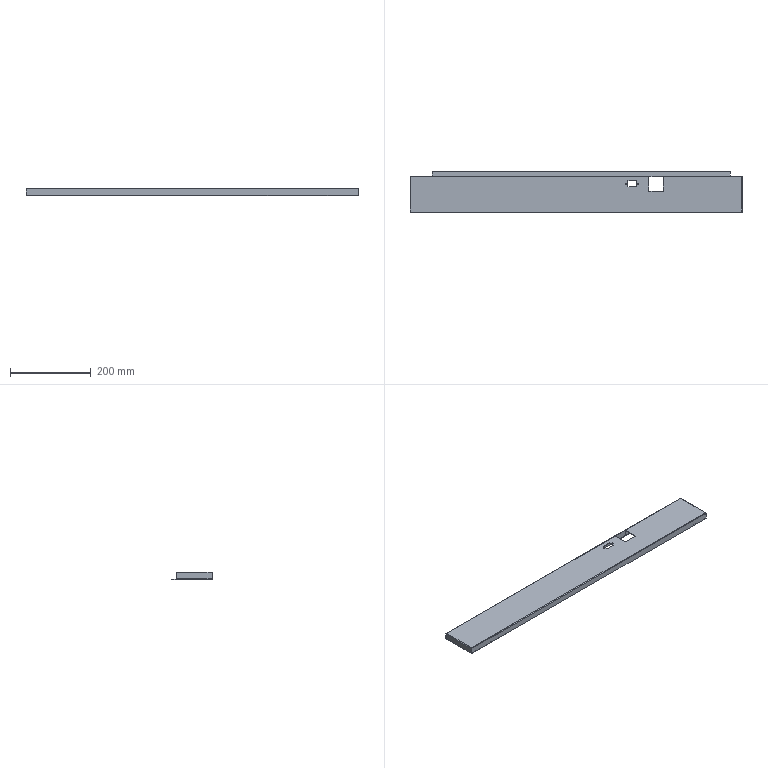Part | NX | features BREP 3 | 3 solids | 100 faces | box 820.5 x 102 x 18 mm | volume 172420 mm3 | plane 81 | cylinder 19 | commonest cylinder face diameters 0.02 x8 3.02 x7 2.5 x4